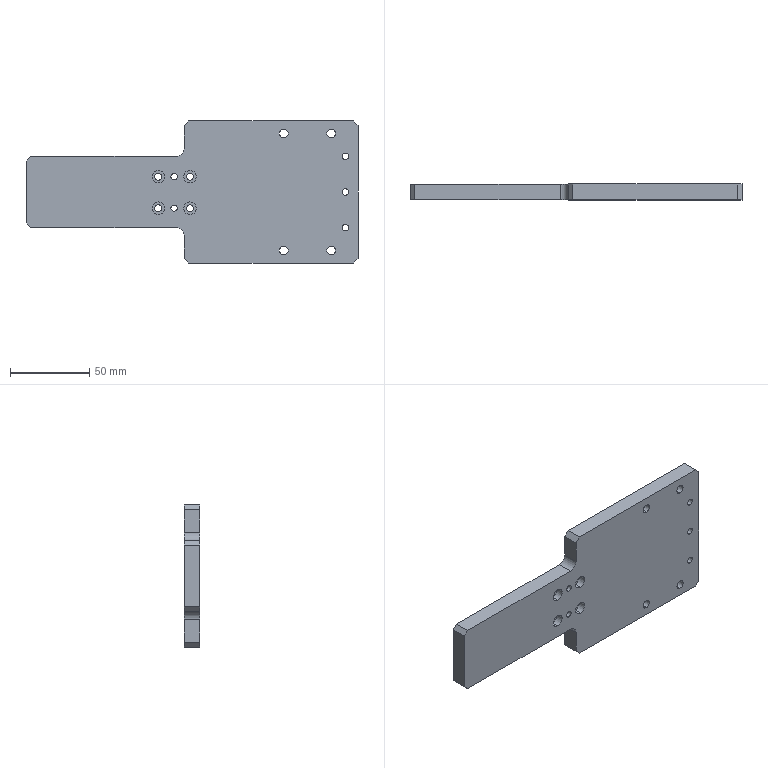Part | SolidWorks | features HoleWzd 4, Chamfer 2, Extrusion 1, Fillet 1, ICE 1 | 1 solid | 68 faces | box 210 x 10 x 90 mm | volume 139703 mm3 | cylinder 44 | plane 24 | commonest cylinder face diameters 10 x10 4.5 x8 5.5 x8 8 x8 4.2 x6 4 x4